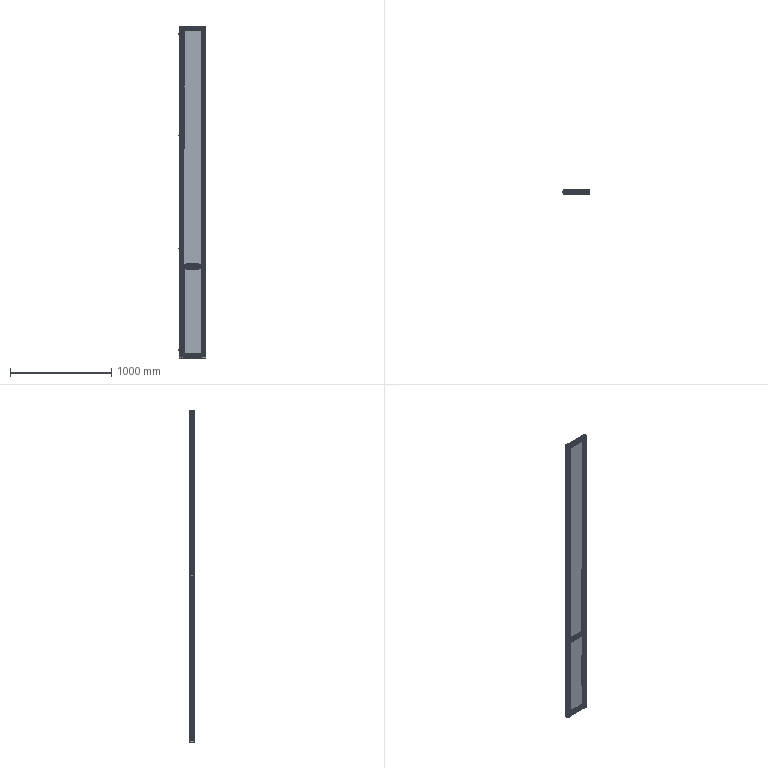Part | SolidWorks | features ReferencePattern 12, LocalLPattern 4 | 67 solids | 3410 faces | volume 7789967 mm3 | plane 2303 | cylinder 935 | cone 140 | spline 32 | commonest cylinder face diameters 0.562 x120 5 x104 6.8 x103 11 x56 2 x54 8 x48